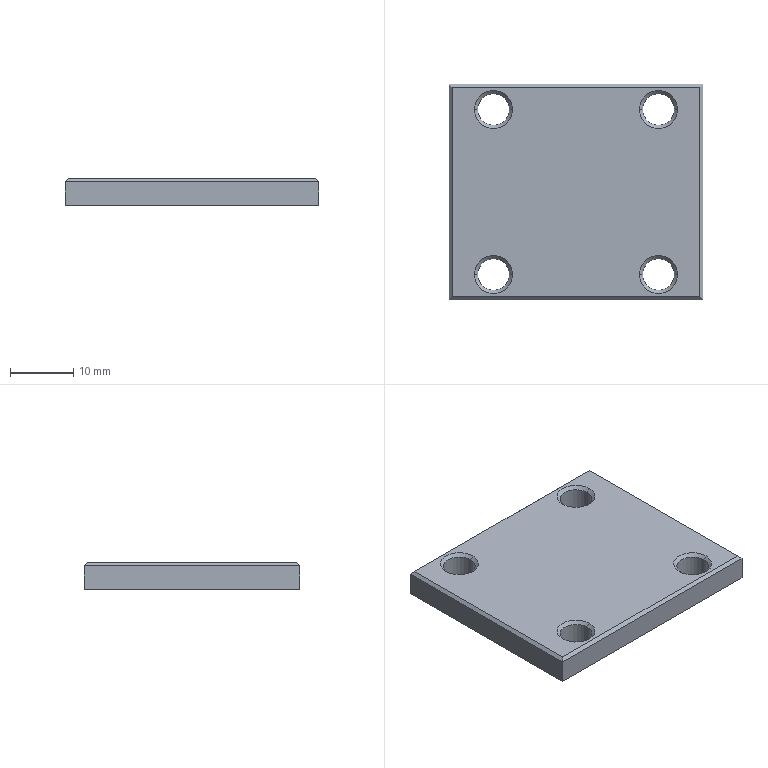Part | NX | 1 solid | 26 faces | box 40 x 34 x 4.25 mm | volume 5419 mm3 | plane 10 | cone 8 | cylinder 8 | commonest cylinder face diameters 5 x8
STEP:
#1=CARTESIAN_POINT('',(30.5,-30.,9.17));
#2=VERTEX_POINT('',#1);
#3=CARTESIAN_POINT('',(35.5,-30.,9.17));
#4=VERTEX_POINT('',#3);
#5=CARTESIAN_POINT('',(33.,-30.,9.17));
#6=DIRECTION('',(0.,0.,1.));
#7=DIRECTION('',(1.,0.,0.));
#8=AXIS2_PLACEMENT_3D('',#5,#6,#7);
#9=CIRCLE('',#8,2.5);
#10=EDGE_CURVE('',#2,#4,#9,.T.);
#11=ORIENTED_EDGE('',*,*,#10,.F.);
#12=CARTESIAN_POINT('',(30.,-30.,9.67));
#13=VERTEX_POINT('',#12);
#14=CARTESIAN_POINT('',(30.,-30.,9.67));
#15=DIRECTION('',(-0.7071,0.,0.7071));
#16=VECTOR('',#15,1000.);
#17=LINE('',#14,#16);
#18=EDGE_CURVE('',#2,#13,#17,.T.);
#19=ORIENTED_EDGE('',*,*,#18,.T.);
#20=CARTESIAN_POINT('',(36.,-30.,9.67));
#21=VERTEX_POINT('',#20);
#22=CARTESIAN_POINT('',(33.,-30.,9.67));
#23=DIRECTION('',(0.,0.,1.));
#24=DIRECTION('',(1.,0.,0.));
#25=AXIS2_PLACEMENT_3D('',#22,#23,#24);
#26=CIRCLE('',#25,3.);
#27=EDGE_CURVE('',#13,#21,#26,.T.);
#28=ORIENTED_EDGE('',*,*,#27,.T.);
#29=CARTESIAN_POINT('',(36.,-30.,9.67));
#30=DIRECTION('',(0.7071,0.,0.7071));
#31=VECTOR('',#30,1000.);
#32=LINE('',#29,#31);
#33=EDGE_CURVE('',#4,#21,#32,.T.);
#34=ORIENTED_EDGE('',*,*,#33,.F.);
#35=EDGE_LOOP('',(#11,#19,#28,#34));
#36=FACE_BOUND('',#35,.T.);
#37=CARTESIAN_POINT('',(33.,-30.,9.67));
#38=DIRECTION('',(0.,0.,1.));
#39=DIRECTION('',(1.,0.,0.));
#40=AXIS2_PLACEMENT_3D('',#37,#38,#39);
#41=CONICAL_SURFACE('',#40,3.,0.7854);
#42=ADVANCED_FACE('',(#36),#41,.F.);
#43=CARTESIAN_POINT('',(0.,0.,9.17));
#44=VERTEX_POINT('',#43);
#45=CARTESIAN_POINT('',(0.,-34.,9.17));
#46=VERTEX_POINT('',#45);
#47=CARTESIAN_POINT('',(0.,0.,9.17));
#48=DIRECTION('',(0.,-1.,0.));
#49=VECTOR('',#48,1000.);
#50=LINE('',#47,#49);
#51=EDGE_CURVE('',#44,#46,#50,.T.);
#52=ORIENTED_EDGE('',*,*,#51,.F.);
#53=CARTESIAN_POINT('',(0.,0.,5.42));
#54=VERTEX_POINT('',#53);
#55=CARTESIAN_POINT('',(0.,0.,0.));
#56=DIRECTION('',(0.,0.,-1.));
#57=VECTOR('',#56,1000.);
#58=LINE('',#55,#57);
#59=EDGE_CURVE('',#44,#54,#58,.T.);
#60=ORIENTED_EDGE('',*,*,#59,.T.);
#61=CARTESIAN_POINT('',(0.,-34.,5.42));
#62=VERTEX_POINT('',#61);
#63=CARTESIAN_POINT('',(0.,0.,5.42));
#64=DIRECTION('',(0.,-1.,0.));
#65=VECTOR('',#64,1000.);
#66=LINE('',#63,#65);
#67=EDGE_CURVE('',#54,#62,#66,.T.);
#68=ORIENTED_EDGE('',*,*,#67,.T.);
#69=CARTESIAN_POINT('',(0.,-34.,0.));
#70=DIRECTION('',(0.,0.,1.));
#71=VECTOR('',#70,1000.);
#72=LINE('',#69,#71);
#73=EDGE_CURVE('',#62,#46,#72,.T.);
#74=ORIENTED_EDGE('',*,*,#73,.T.);
#75=EDGE_LOOP('',(#52,#60,#68,#74));
#76=FACE_BOUND('',#75,.T.);
#77=CARTESIAN_POINT('',(0.,0.,0.));
#78=DIRECTION('',(-1.,0.,0.));
#79=DIRECTION('',(0.,0.,1.));
#80=AXIS2_PLACEMENT_3D('',#77,#78,#79);
#81=PLANE('',#80);
#82=ADVANCED_FACE('',(#76),#81,.T.);
#83=CARTESIAN_POINT('',(40.,0.,9.17));
#84=VERTEX_POINT('',#83);
#85=CARTESIAN_POINT('',(0.,0.,9.17));
#86=DIRECTION('',(1.,0.,0.));
#87=VECTOR('',#86,1000.);
#88=LINE('',#85,#87);
#89=EDGE_CURVE('',#44,#84,#88,.T.);
#90=ORIENTED_EDGE('',*,*,#89,.T.);
#91=CARTESIAN_POINT('',(40.,0.,5.42));
#92=VERTEX_POINT('',#91);
#93=CARTESIAN_POINT('',(40.,0.,0.));
#94=DIRECTION('',(0.,0.,1.));
#95=VECTOR('',#94,1000.);
#96=LINE('',#93,#95);
#97=EDGE_CURVE('',#92,#84,#96,.T.);
#98=ORIENTED_EDGE('',*,*,#97,.F.);
#99=CARTESIAN_POINT('',(0.,0.,5.42));
#100=DIRECTION('',(-1.,0.,0.));
#101=VECTOR('',#100,1000.);
#102=LINE('',#99,#101);
#103=EDGE_CURVE('',#92,#54,#102,.T.);
#104=ORIENTED_EDGE('',*,*,#103,.T.);
#105=ORIENTED_EDGE('',*,*,#59,.F.);
#106=EDGE_LOOP('',(#90,#98,#104,#105));
#107=FACE_BOUND('',#106,.T.);
#108=CARTESIAN_POINT('',(40.,0.,0.));
#109=DIRECTION('',(0.,1.,0.));
#110=DIRECTION('',(1.,0.,0.));
#111=AXIS2_PLACEMENT_3D('',#108,#109,#110);
#112=PLANE('',#111);
#113=ADVANCED_FACE('',(#107),#112,.T.);
#114=CARTESIAN_POINT('',(40.,-34.,9.17));
#115=VERTEX_POINT('',#114);
#116=CARTESIAN_POINT('',(40.,0.,9.17));
#117=DIRECTION('',(0.,1.,0.));
#118=VECTOR('',#117,1000.);
#119=LINE('',#116,#118);
#120=EDGE_CURVE('',#115,#84,#119,.T.);
#121=ORIENTED_EDGE('',*,*,#120,.F.);
#122=CARTESIAN_POINT('',(40.,-34.,5.42));
#123=VERTEX_POINT('',#122);
#124=CARTESIAN_POINT('',(40.,-34.,0.));
#125=DIRECTION('',(0.,0.,-1.));
#126=VECTOR('',#125,1000.);
#127=LINE('',#124,#126);
#128=EDGE_CURVE('',#115,#123,#127,.T.);
#129=ORIENTED_EDGE('',*,*,#128,.T.);
#130=CARTESIAN_POINT('',(40.,0.,5.42));
#131=DIRECTION('',(0.,1.,0.));
#132=VECTOR('',#131,1000.);
#133=LINE('',#130,#132);
#134=EDGE_CURVE('',#123,#92,#133,.T.);
#135=ORIENTED_EDGE('',*,*,#134,.T.);
#136=ORIENTED_EDGE('',*,*,#97,.T.);
#137=EDGE_LOOP('',(#121,#129,#135,#136));
#138=FACE_BOUND('',#137,.T.);
#139=CARTESIAN_POINT('',(40.,-34.,0.));
#140=DIRECTION('',(1.,0.,0.));
#141=DIRECTION('',(0.,1.,0.));
#142=AXIS2_PLACEMENT_3D('',#139,#140,#141);
#143=PLANE('',#142);
#144=ADVANCED_FACE('',(#138),#143,.T.);
#145=CARTESIAN_POINT('',(0.,-34.,9.17));
#146=DIRECTION('',(1.,0.,0.));
#147=VECTOR('',#146,1000.);
#148=LINE('',#145,#147);
#149=EDGE_CURVE('',#46,#115,#148,.T.);
#150=ORIENTED_EDGE('',*,*,#149,.F.);
#151=ORIENTED_EDGE('',*,*,#73,.F.);
#152=CARTESIAN_POINT('',(0.,-34.,5.42));
#153=DIRECTION('',(1.,0.,0.));
#154=VECTOR('',#153,1000.);
#155=LINE('',#152,#154);
#156=EDGE_CURVE('',#62,#123,#155,.T.);
#157=ORIENTED_EDGE('',*,*,#156,.T.);
#158=ORIENTED_EDGE('',*,*,#128,.F.);
#159=EDGE_LOOP('',(#150,#151,#157,#158));
#160=FACE_BOUND('',#159,.T.);
#161=CARTESIAN_POINT('',(0.,-34.,0.));
#162=DIRECTION('',(0.,-1.,0.));
#163=DIRECTION('',(0.,0.,-1.));
#164=AXIS2_PLACEMENT_3D('',#161,#162,#163);
#165=PLANE('',#164);
#166=ADVANCED_FACE('',(#160),#165,.T.);
#167=ORIENTED_EDGE('',*,*,#134,.F.);
#168=ORIENTED_EDGE('',*,*,#156,.F.);
#169=ORIENTED_EDGE('',*,*,#67,.F.);
#170=ORIENTED_EDGE('',*,*,#103,.F.);
#171=EDGE_LOOP('',(#167,#168,#169,#170));
#172=FACE_BOUND('',#171,.T.);
#173=CARTESIAN_POINT('',(30.5,-30.,5.42));
#174=VERTEX_POINT('',#173);
#175=CARTESIAN_POINT('',(35.5,-30.,5.42));
#176=VERTEX_POINT('',#175);
#177=CARTESIAN_POINT('',(33.,-30.,5.42));
#178=DIRECTION('',(0.,0.,-1.));
#179=DIRECTION('',(-1.,0.,0.));
#180=AXIS2_PLACEMENT_3D('',#177,#178,#179);
#181=CIRCLE('',#180,2.5);
#182=EDGE_CURVE('',#174,#176,#181,.T.);
#183=ORIENTED_EDGE('',*,*,#182,.F.);
#184=CARTESIAN_POINT('',(33.,-30.,5.42));
#185=DIRECTION('',(0.,0.,-1.));
#186=DIRECTION('',(-1.,0.,0.));
#187=AXIS2_PLACEMENT_3D('',#184,#185,#186);
#188=CIRCLE('',#187,2.5);
#189=EDGE_CURVE('',#176,#174,#188,.T.);
#190=ORIENTED_EDGE('',*,*,#189,.F.);
#191=EDGE_LOOP('',(#183,#190));
#192=FACE_BOUND('',#191,.T.);
#193=CARTESIAN_POINT('',(4.5,-4.,5.42));
#194=VERTEX_POINT('',#193);
#195=CARTESIAN_POINT('',(9.5,-4.,5.42));
#196=VERTEX_POINT('',#195);
#197=CARTESIAN_POINT('',(7.,-4.,5.42));
#198=DIRECTION('',(0.,0.,-1.));
#199=DIRECTION('',(-1.,0.,0.));
#200=AXIS2_PLACEMENT_3D('',#197,#198,#199);
#201=CIRCLE('',#200,2.5);
#202=EDGE_CURVE('',#194,#196,#201,.T.);
#203=ORIENTED_EDGE('',*,*,#202,.F.);
#204=CARTESIAN_POINT('',(7.,-4.,5.42));
#205=DIRECTION('',(0.,0.,-1.));
#206=DIRECTION('',(-1.,0.,0.));
#207=AXIS2_PLACEMENT_3D('',#204,#205,#206);
#208=CIRCLE('',#207,2.5);
#209=EDGE_CURVE('',#196,#194,#208,.T.);
#210=ORIENTED_EDGE('',*,*,#209,.F.);
#211=EDGE_LOOP('',(#203,#210));
#212=FACE_BOUND('',#211,.T.);
#213=CARTESIAN_POINT('',(30.5,-4.,5.42));
#214=VERTEX_POINT('',#213);
#215=CARTESIAN_POINT('',(35.5,-4.,5.42));
#216=VERTEX_POINT('',#215);
#217=CARTESIAN_POINT('',(33.,-4.,5.42));
#218=DIRECTION('',(0.,0.,-1.));
#219=DIRECTION('',(-1.,0.,0.));
#220=AXIS2_PLACEMENT_3D('',#217,#218,#219);
#221=CIRCLE('',#220,2.5);
#222=EDGE_CURVE('',#214,#216,#221,.T.);
#223=ORIENTED_EDGE('',*,*,#222,.F.);
#224=CARTESIAN_POINT('',(33.,-4.,5.42));
#225=DIRECTION('',(0.,0.,-1.));
#226=DIRECTION('',(-1.,0.,0.));
#227=AXIS2_PLACEMENT_3D('',#224,#225,#226);
#228=CIRCLE('',#227,2.5);
#229=EDGE_CURVE('',#216,#214,#228,.T.);
#230=ORIENTED_EDGE('',*,*,#229,.F.);
#231=EDGE_LOOP('',(#223,#230));
#232=FACE_BOUND('',#231,.T.);
#233=CARTESIAN_POINT('',(9.5,-30.,5.42));
#234=VERTEX_POINT('',#233);
#235=CARTESIAN_POINT('',(4.5,-30.,5.42));
#236=VERTEX_POINT('',#235);
#237=CARTESIAN_POINT('',(7.,-30.,5.42));
#238=DIRECTION('',(0.,0.,-1.));
#239=DIRECTION('',(-1.,0.,0.));
#240=AXIS2_PLACEMENT_3D('',#237,#238,#239);
#241=CIRCLE('',#240,2.5);
#242=EDGE_CURVE('',#234,#236,#241,.T.);
#243=ORIENTED_EDGE('',*,*,#242,.F.);
#244=CARTESIAN_POINT('',(7.,-30.,5.42));
#245=DIRECTION('',(0.,0.,-1.));
#246=DIRECTION('',(-1.,0.,0.));
#247=AXIS2_PLACEMENT_3D('',#244,#245,#246);
#248=CIRCLE('',#247,2.5);
#249=EDGE_CURVE('',#236,#234,#248,.T.);
#250=ORIENTED_EDGE('',*,*,#249,.F.);
#251=EDGE_LOOP('',(#243,#250));
#252=FACE_BOUND('',#251,.T.);
#253=CARTESIAN_POINT('',(0.,0.,5.42));
#254=DIRECTION('',(0.,0.,1.));
#255=DIRECTION('',(1.,0.,0.));
#256=AXIS2_PLACEMENT_3D('',#253,#254,#255);
#257=PLANE('',#256);
#258=ADVANCED_FACE('',(#172,#192,#212,#232,#252),#257,.F.);
#259=ORIENTED_EDGE('',*,*,#202,.T.);
#260=CARTESIAN_POINT('',(9.5,-4.,9.17));
#261=VERTEX_POINT('',#260);
#262=CARTESIAN_POINT('',(9.5,-4.,10.5));
#263=DIRECTION('',(0.,0.,-1.));
#264=VECTOR('',#263,1000.);
#265=LINE('',#262,#264);
#266=EDGE_CURVE('',#261,#196,#265,.T.);
#267=ORIENTED_EDGE('',*,*,#266,.F.);
#268=CARTESIAN_POINT('',(4.5,-4.,9.17));
#269=VERTEX_POINT('',#268);
#270=CARTESIAN_POINT('',(7.,-4.,9.17));
#271=DIRECTION('',(0.,0.,-1.));
#272=DIRECTION('',(-1.,0.,0.));
#273=AXIS2_PLACEMENT_3D('',#270,#271,#272);
#274=CIRCLE('',#273,2.5);
#275=EDGE_CURVE('',#269,#261,#274,.T.);
#276=ORIENTED_EDGE('',*,*,#275,.F.);
#277=CARTESIAN_POINT('',(4.5,-4.,10.5));
#278=DIRECTION('',(0.,0.,-1.));
#279=VECTOR('',#278,1000.);
#280=LINE('',#277,#279);
#281=EDGE_CURVE('',#269,#194,#280,.T.);
#282=ORIENTED_EDGE('',*,*,#281,.T.);
#283=EDGE_LOOP('',(#259,#267,#276,#282));
#284=FACE_BOUND('',#283,.T.);
#285=CARTESIAN_POINT('',(7.,-4.,10.5));
#286=DIRECTION('',(0.,0.,-1.));
#287=DIRECTION('',(-1.,0.,0.));
#288=AXIS2_PLACEMENT_3D('',#285,#286,#287);
#289=CYLINDRICAL_SURFACE('',#288,2.5);
#290=ADVANCED_FACE('',(#284),#289,.F.);
#291=ORIENTED_EDGE('',*,*,#222,.T.);
#292=CARTESIAN_POINT('',(35.5,-4.,9.17));
#293=VERTEX_POINT('',#292);
#294=CARTESIAN_POINT('',(35.5,-4.,10.5));
#295=DIRECTION('',(0.,0.,-1.));
#296=VECTOR('',#295,1000.);
#297=LINE('',#294,#296);
#298=EDGE_CURVE('',#216,#293,#297,.F.);
#299=ORIENTED_EDGE('',*,*,#298,.T.);
#300=CARTESIAN_POINT('',(30.5,-4.,9.17));
#301=VERTEX_POINT('',#300);
#302=CARTESIAN_POINT('',(33.,-4.,9.17));
#303=DIRECTION('',(0.,0.,-1.));
#304=DIRECTION('',(-1.,0.,0.));
#305=AXIS2_PLACEMENT_3D('',#302,#303,#304);
#306=CIRCLE('',#305,2.5);
#307=EDGE_CURVE('',#301,#293,#306,.T.);
#308=ORIENTED_EDGE('',*,*,#307,.F.);
#309=CARTESIAN_POINT('',(30.5,-4.,10.5));
#310=DIRECTION('',(0.,0.,-1.));
#311=VECTOR('',#310,1000.);
#312=LINE('',#309,#311);
#313=EDGE_CURVE('',#214,#301,#312,.F.);
#314=ORIENTED_EDGE('',*,*,#313,.F.);
#315=EDGE_LOOP('',(#291,#299,#308,#314));
#316=FACE_BOUND('',#315,.T.);
#317=CARTESIAN_POINT('',(33.,-4.,10.5));
#318=DIRECTION('',(0.,0.,-1.));
#319=DIRECTION('',(-1.,0.,0.));
#320=AXIS2_PLACEMENT_3D('',#317,#318,#319);
#321=CYLINDRICAL_SURFACE('',#320,2.5);
#322=ADVANCED_FACE('',(#316),#321,.F.);
#323=CARTESIAN_POINT('',(9.5,-30.,9.17));
#324=VERTEX_POINT('',#323);
#325=CARTESIAN_POINT('',(4.5,-30.,9.17));
#326=VERTEX_POINT('',#325);
#327=CARTESIAN_POINT('',(7.,-30.,9.17));
#328=DIRECTION('',(0.,0.,1.));
#329=DIRECTION('',(1.,0.,0.));
#330=AXIS2_PLACEMENT_3D('',#327,#328,#329);
#331=CIRCLE('',#330,2.5);
#332=EDGE_CURVE('',#324,#326,#331,.T.);
#333=ORIENTED_EDGE('',*,*,#332,.T.);
#334=CARTESIAN_POINT('',(4.5,-30.,10.5));
#335=DIRECTION('',(0.,0.,-1.));
#336=VECTOR('',#335,1000.);
#337=LINE('',#334,#336);
#338=EDGE_CURVE('',#236,#326,#337,.F.);
#339=ORIENTED_EDGE('',*,*,#338,.F.);
#340=ORIENTED_EDGE('',*,*,#249,.T.);
#341=CARTESIAN_POINT('',(9.5,-30.,10.5));
#342=DIRECTION('',(0.,0.,-1.));
#343=VECTOR('',#342,1000.);
#344=LINE('',#341,#343);
#345=EDGE_CURVE('',#234,#324,#344,.F.);
#346=ORIENTED_EDGE('',*,*,#345,.T.);
#347=EDGE_LOOP('',(#333,#339,#340,#346));
#348=FACE_BOUND('',#347,.T.);
#349=CARTESIAN_POINT('',(7.,-30.,10.5));
#350=DIRECTION('',(0.,0.,-1.));
#351=DIRECTION('',(-1.,0.,0.));
#352=AXIS2_PLACEMENT_3D('',#349,#350,#351);
#353=CYLINDRICAL_SURFACE('',#352,2.5);
#354=ADVANCED_FACE('',(#348),#353,.F.);
#355=ORIENTED_EDGE('',*,*,#182,.T.);
#356=CARTESIAN_POINT('',(35.5,-30.,10.5));
#357=DIRECTION('',(0.,0.,-1.));
#358=VECTOR('',#357,1000.);
#359=LINE('',#356,#358);
#360=EDGE_CURVE('',#4,#176,#359,.T.);
#361=ORIENTED_EDGE('',*,*,#360,.F.);
#362=CARTESIAN_POINT('',(33.,-30.,9.17));
#363=DIRECTION('',(0.,0.,1.));
#364=DIRECTION('',(1.,0.,0.));
#365=AXIS2_PLACEMENT_3D('',#362,#363,#364);
#366=CIRCLE('',#365,2.5);
#367=EDGE_CURVE('',#4,#2,#366,.T.);
#368=ORIENTED_EDGE('',*,*,#367,.T.);
#369=CARTESIAN_POINT('',(30.5,-30.,10.5));
#370=DIRECTION('',(0.,0.,-1.));
#371=VECTOR('',#370,1000.);
#372=LINE('',#369,#371);
#373=EDGE_CURVE('',#2,#174,#372,.T.);
#374=ORIENTED_EDGE('',*,*,#373,.T.);
#375=EDGE_LOOP('',(#355,#361,#368,#374));
#376=FACE_BOUND('',#375,.T.);
#377=CARTESIAN_POINT('',(33.,-30.,10.5));
#378=DIRECTION('',(0.,0.,-1.));
#379=DIRECTION('',(-1.,0.,0.));
#380=AXIS2_PLACEMENT_3D('',#377,#378,#379);
#381=CYLINDRICAL_SURFACE('',#380,2.5);
#382=ADVANCED_FACE('',(#376),#381,.F.);
#383=ORIENTED_EDGE('',*,*,#120,.T.);
#384=CARTESIAN_POINT('',(39.5,-0.5,9.67));
#385=VERTEX_POINT('',#384);
#386=CARTESIAN_POINT('',(49.17,9.17,0.));
#387=DIRECTION('',(0.5774,0.5774,-0.5774));
#388=VECTOR('',#387,1000.);
#389=LINE('',#386,#388);
#390=EDGE_CURVE('',#385,#84,#389,.T.);
#391=ORIENTED_EDGE('',*,*,#390,.F.);
#392=CARTESIAN_POINT('',(39.5,-33.5,9.67));
#393=VERTEX_POINT('',#392);
#394=CARTESIAN_POINT('',(39.5,0.,9.67));
#395=DIRECTION('',(0.,-1.,0.));
#396=VECTOR('',#395,1000.);
#397=LINE('',#394,#396);
#398=EDGE_CURVE('',#385,#393,#397,.T.);
#399=ORIENTED_EDGE('',*,*,#398,.T.);
#400=CARTESIAN_POINT('',(49.17,-43.17,0.));
#401=DIRECTION('',(-0.5774,0.5774,0.5774));
#402=VECTOR('',#401,1000.);
#403=LINE('',#400,#402);
#404=EDGE_CURVE('',#115,#393,#403,.T.);
#405=ORIENTED_EDGE('',*,*,#404,.F.);
#406=EDGE_LOOP('',(#383,#391,#399,#405));
#407=FACE_BOUND('',#406,.T.);
#408=CARTESIAN_POINT('',(39.75,-17.,9.42));
#409=DIRECTION('',(-0.7071,0.,-0.7071));
#410=DIRECTION('',(-0.7071,0.,0.7071));
#411=AXIS2_PLACEMENT_3D('',#408,#409,#410);
#412=PLANE('',#411);
#413=ADVANCED_FACE('',(#407),#412,.F.);
#414=CARTESIAN_POINT('',(7.,-4.,9.17));
#415=DIRECTION('',(0.,0.,-1.));
#416=DIRECTION('',(-1.,0.,0.));
#417=AXIS2_PLACEMENT_3D('',#414,#415,#416);
#418=CIRCLE('',#417,2.5);
#419=EDGE_CURVE('',#261,#269,#418,.T.);
#420=ORIENTED_EDGE('',*,*,#419,.T.);
#421=CARTESIAN_POINT('',(4.,-4.,9.67));
#422=VERTEX_POINT('',#421);
#423=CARTESIAN_POINT('',(4.,-4.,9.67));
#424=DIRECTION('',(-0.7071,0.,0.7071));
#425=VECTOR('',#424,1000.);
#426=LINE('',#423,#425);
#427=EDGE_CURVE('',#422,#269,#426,.F.);
#428=ORIENTED_EDGE('',*,*,#427,.F.);
#429=CARTESIAN_POINT('',(10.,-4.,9.67));
#430=VERTEX_POINT('',#429);
#431=CARTESIAN_POINT('',(7.,-4.,9.67));
#432=DIRECTION('',(0.,0.,1.));
#433=DIRECTION('',(1.,0.,0.));
#434=AXIS2_PLACEMENT_3D('',#431,#432,#433);
#435=CIRCLE('',#434,3.);
#436=EDGE_CURVE('',#422,#430,#435,.T.);
#437=ORIENTED_EDGE('',*,*,#436,.T.);
#438=CARTESIAN_POINT('',(10.,-4.,9.67));
#439=DIRECTION('',(0.7071,0.,0.7071));
#440=VECTOR('',#439,1000.);
#441=LINE('',#438,#440);
#442=EDGE_CURVE('',#430,#261,#441,.F.);
#443=ORIENTED_EDGE('',*,*,#442,.T.);
#444=EDGE_LOOP('',(#420,#428,#437,#443));
#445=FACE_BOUND('',#444,.T.);
#446=CARTESIAN_POINT('',(7.,-4.,9.67));
#447=DIRECTION('',(0.,0.,1.));
#448=DIRECTION('',(1.,0.,0.));
#449=AXIS2_PLACEMENT_3D('',#446,#447,#448);
#450=CONICAL_SURFACE('',#449,3.,0.7854);
#451=ADVANCED_FACE('',(#445),#450,.F.);
#452=ORIENTED_EDGE('',*,*,#51,.T.);
#453=CARTESIAN_POINT('',(0.5,-33.5,9.67));
#454=VERTEX_POINT('',#453);
#455=CARTESIAN_POINT('',(-9.17,-43.17,0.));
#456=DIRECTION('',(-0.5774,-0.5774,-0.5774));
#457=VECTOR('',#456,1000.);
#458=LINE('',#455,#457);
#459=EDGE_CURVE('',#454,#46,#458,.T.);
#460=ORIENTED_EDGE('',*,*,#459,.F.);
#461=CARTESIAN_POINT('',(0.5,-0.5,9.67));
#462=VERTEX_POINT('',#461);
#463=CARTESIAN_POINT('',(0.5,0.,9.67));
#464=DIRECTION('',(0.,-1.,0.));
#465=VECTOR('',#464,1000.);
#466=LINE('',#463,#465);
#467=EDGE_CURVE('',#462,#454,#466,.T.);
#468=ORIENTED_EDGE('',*,*,#467,.F.);
#469=CARTESIAN_POINT('',(-9.17,9.17,0.));
#470=DIRECTION('',(0.5774,-0.5774,0.5774));
#471=VECTOR('',#470,1000.);
#472=LINE('',#469,#471);
#473=EDGE_CURVE('',#44,#462,#472,.T.);
#474=ORIENTED_EDGE('',*,*,#473,.F.);
#475=EDGE_LOOP('',(#452,#460,#468,#474));
#476=FACE_BOUND('',#475,.T.);
#477=CARTESIAN_POINT('',(0.25,-17.,9.42));
#478=DIRECTION('',(0.7071,0.,-0.7071));
#479=DIRECTION('',(0.,-1.,0.));
#480=AXIS2_PLACEMENT_3D('',#477,#478,#479);
#481=PLANE('',#480);
#482=ADVANCED_FACE('',(#476),#481,.F.);
#483=ORIENTED_EDGE('',*,*,#89,.F.);
#484=ORIENTED_EDGE('',*,*,#473,.T.);
#485=CARTESIAN_POINT('',(0.,-0.5,9.67));
#486=DIRECTION('',(-1.,0.,0.));
#487=VECTOR('',#486,1000.);
#488=LINE('',#485,#487);
#489=EDGE_CURVE('',#385,#462,#488,.T.);
#490=ORIENTED_EDGE('',*,*,#489,.F.);
#491=ORIENTED_EDGE('',*,*,#390,.T.);
#492=EDGE_LOOP('',(#483,#484,#490,#491));
#493=FACE_BOUND('',#492,.T.);
#494=CARTESIAN_POINT('',(20.,-0.25,9.42));
#495=DIRECTION('',(0.,0.7071,0.7071));
#496=DIRECTION('',(1.,0.,0.));
#497=AXIS2_PLACEMENT_3D('',#494,#495,#496);
#498=PLANE('',#497);
#499=ADVANCED_FACE('',(#493),#498,.T.);
#500=ORIENTED_EDGE('',*,*,#149,.T.);
#501=ORIENTED_EDGE('',*,*,#404,.T.);
#502=CARTESIAN_POINT('',(0.,-33.5,9.67));
#503=DIRECTION('',(1.,0.,0.));
#504=VECTOR('',#503,1000.);
#505=LINE('',#502,#504);
#506=EDGE_CURVE('',#454,#393,#505,.T.);
#507=ORIENTED_EDGE('',*,*,#506,.F.);
#508=ORIENTED_EDGE('',*,*,#459,.T.);
#509=EDGE_LOOP('',(#500,#501,#507,#508));
#510=FACE_BOUND('',#509,.T.);
#511=CARTESIAN_POINT('',(20.,-33.75,9.42));
#512=DIRECTION('',(0.,-0.7071,0.7071));
#513=DIRECTION('',(-1.,0.,0.));
#514=AXIS2_PLACEMENT_3D('',#511,#512,#513);
#515=PLANE('',#514);
#516=ADVANCED_FACE('',(#510),#515,.T.);
#517=ORIENTED_EDGE('',*,*,#307,.T.);
#518=CARTESIAN_POINT('',(36.,-4.,9.67));
#519=VERTEX_POINT('',#518);
#520=CARTESIAN_POINT('',(36.,-4.,9.67));
#521=DIRECTION('',(0.7071,0.,0.7071));
#522=VECTOR('',#521,1000.);
#523=LINE('',#520,#522);
#524=EDGE_CURVE('',#293,#519,#523,.T.);
#525=ORIENTED_EDGE('',*,*,#524,.T.);
#526=CARTESIAN_POINT('',(30.,-4.,9.67));
#527=VERTEX_POINT('',#526);
#528=CARTESIAN_POINT('',(33.,-4.,9.67));
#529=DIRECTION('',(0.,0.,1.));
#530=DIRECTION('',(1.,0.,0.));
#531=AXIS2_PLACEMENT_3D('',#528,#529,#530);
#532=CIRCLE('',#531,3.);
#533=EDGE_CURVE('',#519,#527,#532,.T.);
#534=ORIENTED_EDGE('',*,*,#533,.T.);
#535=CARTESIAN_POINT('',(30.,-4.,9.67));
#536=DIRECTION('',(-0.7071,0.,0.7071));
#537=VECTOR('',#536,1000.);
#538=LINE('',#535,#537);
#539=EDGE_CURVE('',#301,#527,#538,.T.);
#540=ORIENTED_EDGE('',*,*,#539,.F.);
#541=EDGE_LOOP('',(#517,#525,#534,#540));
#542=FACE_BOUND('',#541,.T.);
#543=CARTESIAN_POINT('',(33.,-4.,9.67));
#544=DIRECTION('',(0.,0.,1.));
#545=DIRECTION('',(1.,0.,0.));
#546=AXIS2_PLACEMENT_3D('',#543,#544,#545);
#547=CONICAL_SURFACE('',#546,3.,0.7854);
#548=ADVANCED_FACE('',(#542),#547,.F.);
#549=CARTESIAN_POINT('',(4.,-30.,9.67));
#550=VERTEX_POINT('',#549);
#551=CARTESIAN_POINT('',(10.,-30.,9.67));
#552=VERTEX_POINT('',#551);
#553=CARTESIAN_POINT('',(7.,-30.,9.67));
#554=DIRECTION('',(0.,0.,1.));
#555=DIRECTION('',(1.,0.,0.));
#556=AXIS2_PLACEMENT_3D('',#553,#554,#555);
#557=CIRCLE('',#556,3.);
#558=EDGE_CURVE('',#550,#552,#557,.T.);
#559=ORIENTED_EDGE('',*,*,#558,.T.);
#560=CARTESIAN_POINT('',(10.,-30.,9.67));
#561=DIRECTION('',(0.7071,0.,0.7071));
#562=VECTOR('',#561,1000.);
#563=LINE('',#560,#562);
#564=EDGE_CURVE('',#324,#552,#563,.T.);
#565=ORIENTED_EDGE('',*,*,#564,.F.);
#566=CARTESIAN_POINT('',(7.,-30.,9.17));
#567=DIRECTION('',(0.,0.,1.));
#568=DIRECTION('',(1.,0.,0.));
#569=AXIS2_PLACEMENT_3D('',#566,#567,#568);
#570=CIRCLE('',#569,2.5);
#571=EDGE_CURVE('',#326,#324,#570,.T.);
#572=ORIENTED_EDGE('',*,*,#571,.F.);
#573=CARTESIAN_POINT('',(4.,-30.,9.67));
#574=DIRECTION('',(-0.7071,0.,0.7071));
#575=VECTOR('',#574,1000.);
#576=LINE('',#573,#575);
#577=EDGE_CURVE('',#326,#550,#576,.T.);
#578=ORIENTED_EDGE('',*,*,#577,.T.);
#579=EDGE_LOOP('',(#559,#565,#572,#578));
#580=FACE_BOUND('',#579,.T.);
#581=CARTESIAN_POINT('',(7.,-30.,9.67));
#582=DIRECTION('',(0.,0.,1.));
#583=DIRECTION('',(1.,0.,0.));
#584=AXIS2_PLACEMENT_3D('',#581,#582,#583);
#585=CONICAL_SURFACE('',#584,3.,0.7854);
#586=ADVANCED_FACE('',(#580),#585,.F.);
#587=ORIENTED_EDGE('',*,*,#467,.T.);
#588=ORIENTED_EDGE('',*,*,#506,.T.);
#589=ORIENTED_EDGE('',*,*,#398,.F.);
#590=ORIENTED_EDGE('',*,*,#489,.T.);
#591=EDGE_LOOP('',(#587,#588,#589,#590));
#592=FACE_BOUND('',#591,.T.);
#593=CARTESIAN_POINT('',(7.,-4.,9.67));
#594=DIRECTION('',(0.,0.,1.));
#595=DIRECTION('',(1.,0.,0.));
#596=AXIS2_PLACEMENT_3D('',#593,#594,#595);
#597=CIRCLE('',#596,3.);
#598=EDGE_CURVE('',#430,#422,#597,.T.);
#599=ORIENTED_EDGE('',*,*,#598,.F.);
#600=ORIENTED_EDGE('',*,*,#436,.F.);
#601=EDGE_LOOP('',(#599,#600));
#602=FACE_BOUND('',#601,.T.);
#603=ORIENTED_EDGE('',*,*,#27,.F.);
#604=CARTESIAN_POINT('',(33.,-30.,9.67));
#605=DIRECTION('',(0.,0.,1.));
#606=DIRECTION('',(1.,0.,0.));
#607=AXIS2_PLACEMENT_3D('',#604,#605,#606);
#608=CIRCLE('',#607,3.);
#609=EDGE_CURVE('',#21,#13,#608,.T.);
#610=ORIENTED_EDGE('',*,*,#609,.F.);
#611=EDGE_LOOP('',(#603,#610));
#612=FACE_BOUND('',#611,.T.);
#613=ORIENTED_EDGE('',*,*,#533,.F.);
#614=CARTESIAN_POINT('',(33.,-4.,9.67));
#615=DIRECTION('',(0.,0.,1.));
#616=DIRECTION('',(1.,0.,0.));
#617=AXIS2_PLACEMENT_3D('',#614,#615,#616);
#618=CIRCLE('',#617,3.);
#619=EDGE_CURVE('',#527,#519,#618,.T.);
#620=ORIENTED_EDGE('',*,*,#619,.F.);
#621=EDGE_LOOP('',(#613,#620));
#622=FACE_BOUND('',#621,.T.);
#623=ORIENTED_EDGE('',*,*,#558,.F.);
#624=CARTESIAN_POINT('',(7.,-30.,9.67));
#625=DIRECTION('',(0.,0.,1.));
#626=DIRECTION('',(1.,0.,0.));
#627=AXIS2_PLACEMENT_3D('',#624,#625,#626);
#628=CIRCLE('',#627,3.);
#629=EDGE_CURVE('',#552,#550,#628,.T.);
#630=ORIENTED_EDGE('',*,*,#629,.F.);
#631=EDGE_LOOP('',(#623,#630));
#632=FACE_BOUND('',#631,.T.);
#633=CARTESIAN_POINT('',(0.,0.,9.67));
#634=DIRECTION('',(0.,0.,1.));
#635=DIRECTION('',(1.,0.,0.));
#636=AXIS2_PLACEMENT_3D('',#633,#634,#635);
#637=PLANE('',#636);
#638=ADVANCED_FACE('',(#592,#602,#612,#622,#632),#637,.T.);
#639=ORIENTED_EDGE('',*,*,#313,.T.);
#640=CARTESIAN_POINT('',(33.,-4.,9.17));
#641=DIRECTION('',(0.,0.,-1.));
#642=DIRECTION('',(-1.,0.,0.));
#643=AXIS2_PLACEMENT_3D('',#640,#641,#642);
#644=CIRCLE('',#643,2.5);
#645=EDGE_CURVE('',#293,#301,#644,.T.);
#646=ORIENTED_EDGE('',*,*,#645,.F.);
#647=ORIENTED_EDGE('',*,*,#298,.F.);
#648=ORIENTED_EDGE('',*,*,#229,.T.);
#649=EDGE_LOOP('',(#639,#646,#647,#648));
#650=FACE_BOUND('',#649,.T.);
#651=CARTESIAN_POINT('',(33.,-4.,10.5));
#652=DIRECTION('',(0.,0.,-1.));
#653=DIRECTION('',(-1.,0.,0.));
#654=AXIS2_PLACEMENT_3D('',#651,#652,#653);
#655=CYLINDRICAL_SURFACE('',#654,2.5);
#656=ADVANCED_FACE('',(#650),#655,.F.);
#657=ORIENTED_EDGE('',*,*,#524,.F.);
#658=ORIENTED_EDGE('',*,*,#645,.T.);
#659=ORIENTED_EDGE('',*,*,#539,.T.);
#660=ORIENTED_EDGE('',*,*,#619,.T.);
#661=EDGE_LOOP('',(#657,#658,#659,#660));
#662=FACE_BOUND('',#661,.T.);
#663=CARTESIAN_POINT('',(33.,-4.,9.67));
#664=DIRECTION('',(0.,0.,1.));
#665=DIRECTION('',(1.,0.,0.));
#666=AXIS2_PLACEMENT_3D('',#663,#664,#665);
#667=CONICAL_SURFACE('',#666,3.,0.7854);
#668=ADVANCED_FACE('',(#662),#667,.F.);
#669=ORIENTED_EDGE('',*,*,#419,.F.);
#670=ORIENTED_EDGE('',*,*,#266,.T.);
#671=ORIENTED_EDGE('',*,*,#209,.T.);
#672=ORIENTED_EDGE('',*,*,#281,.F.);
#673=EDGE_LOOP('',(#669,#670,#671,#672));
#674=FACE_BOUND('',#673,.T.);
#675=CARTESIAN_POINT('',(7.,-4.,10.5));
#676=DIRECTION('',(0.,0.,-1.));
#677=DIRECTION('',(-1.,0.,0.));
#678=AXIS2_PLACEMENT_3D('',#675,#676,#677);
#679=CYLINDRICAL_SURFACE('',#678,2.5);
#680=ADVANCED_FACE('',(#674),#679,.F.);
#681=ORIENTED_EDGE('',*,*,#598,.T.);
#682=ORIENTED_EDGE('',*,*,#427,.T.);
#683=ORIENTED_EDGE('',*,*,#275,.T.);
#684=ORIENTED_EDGE('',*,*,#442,.F.);
#685=EDGE_LOOP('',(#681,#682,#683,#684));
#686=FACE_BOUND('',#685,.T.);
#687=CARTESIAN_POINT('',(7.,-4.,9.67));
#688=DIRECTION('',(0.,0.,1.));
#689=DIRECTION('',(1.,0.,0.));
#690=AXIS2_PLACEMENT_3D('',#687,#688,#689);
#691=CONICAL_SURFACE('',#690,3.,0.7854);
#692=ADVANCED_FACE('',(#686),#691,.F.);
#693=ORIENTED_EDGE('',*,*,#10,.T.);
#694=ORIENTED_EDGE('',*,*,#360,.T.);
#695=ORIENTED_EDGE('',*,*,#189,.T.);
#696=ORIENTED_EDGE('',*,*,#373,.F.);
#697=EDGE_LOOP('',(#693,#694,#695,#696));
#698=FACE_BOUND('',#697,.T.);
#699=CARTESIAN_POINT('',(33.,-30.,10.5));
#700=DIRECTION('',(0.,0.,-1.));
#701=DIRECTION('',(-1.,0.,0.));
#702=AXIS2_PLACEMENT_3D('',#699,#700,#701);
#703=CYLINDRICAL_SURFACE('',#702,2.5);
#704=ADVANCED_FACE('',(#698),#703,.F.);
#705=ORIENTED_EDGE('',*,*,#242,.T.);
#706=ORIENTED_EDGE('',*,*,#338,.T.);
#707=ORIENTED_EDGE('',*,*,#571,.T.);
#708=ORIENTED_EDGE('',*,*,#345,.F.);
#709=EDGE_LOOP('',(#705,#706,#707,#708));
#710=FACE_BOUND('',#709,.T.);
#711=CARTESIAN_POINT('',(7.,-30.,10.5));
#712=DIRECTION('',(0.,0.,-1.));
#713=DIRECTION('',(-1.,0.,0.));
#714=AXIS2_PLACEMENT_3D('',#711,#712,#713);
#715=CYLINDRICAL_SURFACE('',#714,2.5);
#716=ADVANCED_FACE('',(#710),#715,.F.);
#717=ORIENTED_EDGE('',*,*,#332,.F.);
#718=ORIENTED_EDGE('',*,*,#564,.T.);
#719=ORIENTED_EDGE('',*,*,#629,.T.);
#720=ORIENTED_EDGE('',*,*,#577,.F.);
#721=EDGE_LOOP('',(#717,#718,#719,#720));
#722=FACE_BOUND('',#721,.T.);
#723=CARTESIAN_POINT('',(7.,-30.,9.67));
#724=DIRECTION('',(0.,0.,1.));
#725=DIRECTION('',(1.,0.,0.));
#726=AXIS2_PLACEMENT_3D('',#723,#724,#725);
#727=CONICAL_SURFACE('',#726,3.,0.7854);
#728=ADVANCED_FACE('',(#722),#727,.F.);
#729=ORIENTED_EDGE('',*,*,#33,.T.);
#730=ORIENTED_EDGE('',*,*,#609,.T.);
#731=ORIENTED_EDGE('',*,*,#18,.F.);
#732=ORIENTED_EDGE('',*,*,#367,.F.);
#733=EDGE_LOOP('',(#729,#730,#731,#732));
#734=FACE_BOUND('',#733,.T.);
#735=CARTESIAN_POINT('',(33.,-30.,9.67));
#736=DIRECTION('',(0.,0.,1.));
#737=DIRECTION('',(1.,0.,0.));
#738=AXIS2_PLACEMENT_3D('',#735,#736,#737);
#739=CONICAL_SURFACE('',#738,3.,0.7854);
#740=ADVANCED_FACE('',(#734),#739,.F.);
#741=CLOSED_SHELL('',(#42,#82,#113,#144,#166,#258,#290,#322,#354,#382,#413,#451,#482,#499,#516,#548,#586,#638,#656,#668,#680,#692,#704,#716,#728,#740));
#742=MANIFOLD_SOLID_BREP('',#741);
#743=(LENGTH_UNIT()NAMED_UNIT(*)SI_UNIT(.MILLI.,.METRE.));
#744=UNCERTAINTY_MEASURE_WITH_UNIT(LENGTH_MEASURE(0.00001),#743,'','');
#745=(NAMED_UNIT(*)PLANE_ANGLE_UNIT()SI_UNIT($,.RADIAN.));
#746=(NAMED_UNIT(*)SI_UNIT($,.STERADIAN.)SOLID_ANGLE_UNIT());
#747=(GEOMETRIC_REPRESENTATION_CONTEXT(3)GLOBAL_UNCERTAINTY_ASSIGNED_CONTEXT((#744))GLOBAL_UNIT_ASSIGNED_CONTEXT((#743,#745,#746))REPRESENTATION_CONTEXT('',''));
#748=ADVANCED_BREP_SHAPE_REPRESENTATION('',(#742),#747);